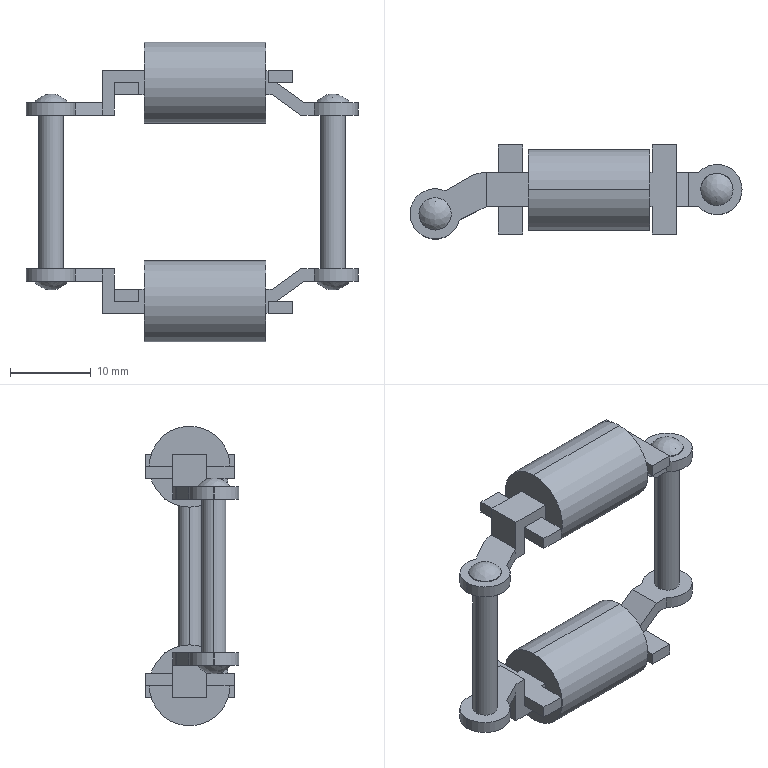Part | SolidWorks | features BaseBody 1 | 1 solid | 100 faces | box 40.999 x 11.6 x 37 mm | volume 3295 mm3 | plane 70 | cylinder 26 | sphere 4 | commonest cylinder face diameters 4 x8 6.2 x8 3 x4 10 x4 8 x2